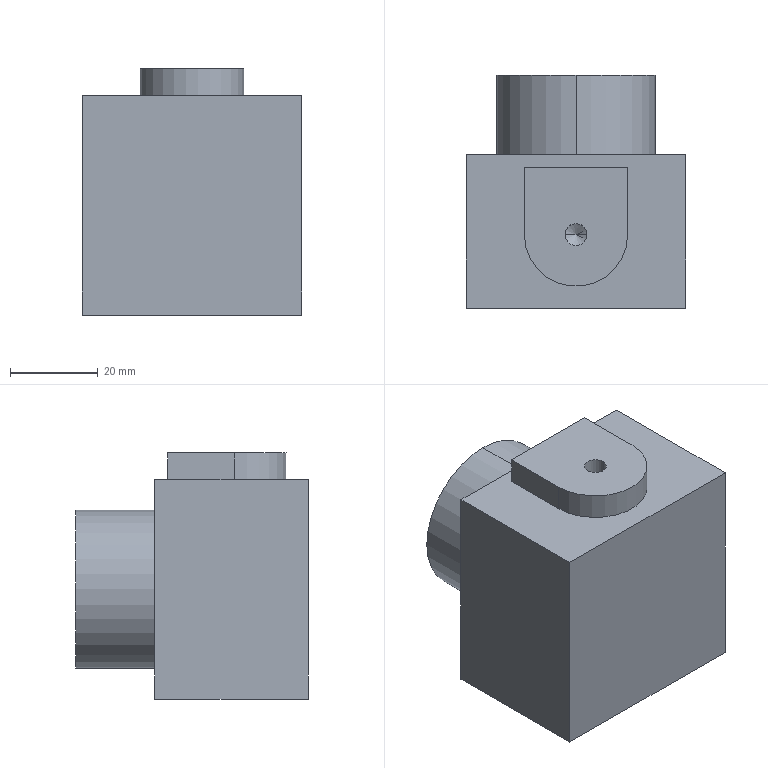Part | SolidWorks | features ICE 2, Extrusion 1, HoleWzd 1 | 1 solid | 18 faces | box 50 x 53 x 56 mm | volume 108930 mm3 | plane 11 | cylinder 5 | cone 2 | commonest cylinder face diameters 5 x2 36 x2 23.5 x1
STEP:
#1=CARTESIAN_POINT('',(-2.5,16.75,14.));
#2=VERTEX_POINT('',#1);
#3=CARTESIAN_POINT('',(2.5,16.75,14.));
#4=VERTEX_POINT('',#3);
#5=CARTESIAN_POINT('',(0.,16.75,14.));
#6=DIRECTION('',(0.,0.,1.));
#7=DIRECTION('',(1.,0.,0.));
#8=AXIS2_PLACEMENT_3D('',#5,#6,#7);
#9=CIRCLE('',#8,2.5);
#10=EDGE_CURVE('',#2,#4,#9,.T.);
#11=ORIENTED_EDGE('',*,*,#10,.F.);
#12=CARTESIAN_POINT('',(-2.5,16.75,31.));
#13=VERTEX_POINT('',#12);
#14=CARTESIAN_POINT('',(-2.5,16.75,31.));
#15=DIRECTION('',(0.,0.,1.));
#16=VECTOR('',#15,1000.);
#17=LINE('',#14,#16);
#18=EDGE_CURVE('',#2,#13,#17,.T.);
#19=ORIENTED_EDGE('',*,*,#18,.T.);
#20=CARTESIAN_POINT('',(2.5,16.75,31.));
#21=VERTEX_POINT('',#20);
#22=CARTESIAN_POINT('',(0.,16.75,31.));
#23=DIRECTION('',(0.,0.,1.));
#24=DIRECTION('',(1.,0.,0.));
#25=AXIS2_PLACEMENT_3D('',#22,#23,#24);
#26=CIRCLE('',#25,2.5);
#27=EDGE_CURVE('',#13,#21,#26,.T.);
#28=ORIENTED_EDGE('',*,*,#27,.T.);
#29=CARTESIAN_POINT('',(2.5,16.75,31.));
#30=DIRECTION('',(0.,0.,1.));
#31=VECTOR('',#30,1000.);
#32=LINE('',#29,#31);
#33=EDGE_CURVE('',#4,#21,#32,.T.);
#34=ORIENTED_EDGE('',*,*,#33,.F.);
#35=EDGE_LOOP('',(#11,#19,#28,#34));
#36=FACE_OUTER_BOUND('',#35,.T.);
#37=CARTESIAN_POINT('',(0.,16.75,31.));
#38=DIRECTION('',(0.,0.,1.));
#39=DIRECTION('',(1.,0.,0.));
#40=AXIS2_PLACEMENT_3D('',#37,#38,#39);
#41=CYLINDRICAL_SURFACE('',#40,2.5);
#42=ADVANCED_FACE('',(#36),#41,.F.);
#43=CARTESIAN_POINT('',(0.,16.75,12.498));
#44=VERTEX_POINT('',#43);
#45=CARTESIAN_POINT('',(2.5,16.75,14.));
#46=DIRECTION('',(0.8572,0.,0.515));
#47=VECTOR('',#46,1000.);
#48=LINE('',#45,#47);
#49=EDGE_CURVE('',#44,#4,#48,.T.);
#50=ORIENTED_EDGE('',*,*,#49,.F.);
#51=CARTESIAN_POINT('',(-2.5,16.75,14.));
#52=DIRECTION('',(-0.8572,0.,0.515));
#53=VECTOR('',#52,1000.);
#54=LINE('',#51,#53);
#55=EDGE_CURVE('',#44,#2,#54,.T.);
#56=ORIENTED_EDGE('',*,*,#55,.T.);
#57=ORIENTED_EDGE('',*,*,#10,.T.);
#58=EDGE_LOOP('',(#50,#56,#57));
#59=FACE_OUTER_BOUND('',#58,.T.);
#60=CARTESIAN_POINT('',(0.,16.75,14.));
#61=DIRECTION('',(0.,0.,1.));
#62=DIRECTION('',(1.,0.,0.));
#63=AXIS2_PLACEMENT_3D('',#60,#61,#62);
#64=CONICAL_SURFACE('',#63,2.5,1.03);
#65=ADVANCED_FACE('',(#59),#64,.F.);
#66=CARTESIAN_POINT('',(0.,53.,18.));
#67=VERTEX_POINT('',#66);
#68=CARTESIAN_POINT('',(0.,53.,-18.));
#69=VERTEX_POINT('',#68);
#70=CARTESIAN_POINT('',(0.,53.,0.));
#71=DIRECTION('',(0.,1.,0.));
#72=DIRECTION('',(0.,0.,1.));
#73=AXIS2_PLACEMENT_3D('',#70,#71,#72);
#74=CIRCLE('',#73,18.);
#75=EDGE_CURVE('',#67,#69,#74,.T.);
#76=ORIENTED_EDGE('',*,*,#75,.F.);
#77=CARTESIAN_POINT('',(0.,35.,18.));
#78=VERTEX_POINT('',#77);
#79=CARTESIAN_POINT('',(0.,53.,18.));
#80=DIRECTION('',(0.,-1.,0.));
#81=VECTOR('',#80,1000.);
#82=LINE('',#79,#81);
#83=EDGE_CURVE('',#67,#78,#82,.T.);
#84=ORIENTED_EDGE('',*,*,#83,.T.);
#85=CARTESIAN_POINT('',(0.,35.,-18.));
#86=VERTEX_POINT('',#85);
#87=CARTESIAN_POINT('',(0.,35.,0.));
#88=DIRECTION('',(0.,1.,0.));
#89=DIRECTION('',(0.,0.,1.));
#90=AXIS2_PLACEMENT_3D('',#87,#88,#89);
#91=CIRCLE('',#90,18.);
#92=EDGE_CURVE('',#78,#86,#91,.T.);
#93=ORIENTED_EDGE('',*,*,#92,.T.);
#94=CARTESIAN_POINT('',(0.,53.,-18.));
#95=DIRECTION('',(0.,-1.,0.));
#96=VECTOR('',#95,1000.);
#97=LINE('',#94,#96);
#98=EDGE_CURVE('',#69,#86,#97,.T.);
#99=ORIENTED_EDGE('',*,*,#98,.F.);
#100=EDGE_LOOP('',(#76,#84,#93,#99));
#101=FACE_OUTER_BOUND('',#100,.T.);
#102=CARTESIAN_POINT('',(0.,53.,0.));
#103=DIRECTION('',(0.,-1.,0.));
#104=DIRECTION('',(0.,0.,-1.));
#105=AXIS2_PLACEMENT_3D('',#102,#103,#104);
#106=CYLINDRICAL_SURFACE('',#105,18.);
#107=ADVANCED_FACE('',(#101),#106,.T.);
#108=CARTESIAN_POINT('',(-25.,0.,25.));
#109=VERTEX_POINT('',#108);
#110=CARTESIAN_POINT('',(25.,0.,25.));
#111=VERTEX_POINT('',#110);
#112=CARTESIAN_POINT('',(-25.,0.,25.));
#113=DIRECTION('',(1.,0.,0.));
#114=VECTOR('',#113,1000.);
#115=LINE('',#112,#114);
#116=EDGE_CURVE('',#109,#111,#115,.T.);
#117=ORIENTED_EDGE('',*,*,#116,.T.);
#118=CARTESIAN_POINT('',(25.,35.,25.));
#119=VERTEX_POINT('',#118);
#120=CARTESIAN_POINT('',(25.,35.,25.));
#121=DIRECTION('',(0.,-1.,0.));
#122=VECTOR('',#121,1000.);
#123=LINE('',#120,#122);
#124=EDGE_CURVE('',#119,#111,#123,.T.);
#125=ORIENTED_EDGE('',*,*,#124,.F.);
#126=CARTESIAN_POINT('',(-25.,35.,25.));
#127=VERTEX_POINT('',#126);
#128=CARTESIAN_POINT('',(-25.,35.,25.));
#129=DIRECTION('',(1.,0.,0.));
#130=VECTOR('',#129,1000.);
#131=LINE('',#128,#130);
#132=EDGE_CURVE('',#127,#119,#131,.T.);
#133=ORIENTED_EDGE('',*,*,#132,.F.);
#134=CARTESIAN_POINT('',(-25.,35.,25.));
#135=DIRECTION('',(0.,-1.,0.));
#136=VECTOR('',#135,1000.);
#137=LINE('',#134,#136);
#138=EDGE_CURVE('',#127,#109,#137,.T.);
#139=ORIENTED_EDGE('',*,*,#138,.T.);
#140=EDGE_LOOP('',(#117,#125,#133,#139));
#141=FACE_OUTER_BOUND('',#140,.T.);
#142=CARTESIAN_POINT('',(-11.75,16.75,25.));
#143=VERTEX_POINT('',#142);
#144=CARTESIAN_POINT('',(11.75,16.75,25.));
#145=VERTEX_POINT('',#144);
#146=CARTESIAN_POINT('',(0.,16.75,25.));
#147=DIRECTION('',(0.,0.,1.));
#148=DIRECTION('',(-1.,0.,0.));
#149=AXIS2_PLACEMENT_3D('',#146,#147,#148);
#150=CIRCLE('',#149,11.75);
#151=EDGE_CURVE('',#143,#145,#150,.T.);
#152=ORIENTED_EDGE('',*,*,#151,.F.);
#153=CARTESIAN_POINT('',(-11.75,32.,25.));
#154=VERTEX_POINT('',#153);
#155=CARTESIAN_POINT('',(-11.75,32.,25.));
#156=DIRECTION('',(0.,-1.,0.));
#157=VECTOR('',#156,1000.);
#158=LINE('',#155,#157);
#159=EDGE_CURVE('',#154,#143,#158,.T.);
#160=ORIENTED_EDGE('',*,*,#159,.F.);
#161=CARTESIAN_POINT('',(11.75,32.,25.));
#162=VERTEX_POINT('',#161);
#163=CARTESIAN_POINT('',(11.75,32.,25.));
#164=DIRECTION('',(-1.,0.,0.));
#165=VECTOR('',#164,1000.);
#166=LINE('',#163,#165);
#167=EDGE_CURVE('',#162,#154,#166,.T.);
#168=ORIENTED_EDGE('',*,*,#167,.F.);
#169=CARTESIAN_POINT('',(11.75,32.,25.));
#170=DIRECTION('',(0.,1.,0.));
#171=VECTOR('',#170,1000.);
#172=LINE('',#169,#171);
#173=EDGE_CURVE('',#145,#162,#172,.T.);
#174=ORIENTED_EDGE('',*,*,#173,.F.);
#175=EDGE_LOOP('',(#152,#160,#168,#174));
#176=FACE_BOUND('',#175,.T.);
#177=CARTESIAN_POINT('',(-25.,35.,25.));
#178=DIRECTION('',(0.,0.,-1.));
#179=DIRECTION('',(-1.,0.,0.));
#180=AXIS2_PLACEMENT_3D('',#177,#178,#179);
#181=PLANE('',#180);
#182=ADVANCED_FACE('',(#141,#176),#181,.F.);
#183=CARTESIAN_POINT('',(25.,0.,-25.));
#184=VERTEX_POINT('',#183);
#185=CARTESIAN_POINT('',(25.,0.,25.));
#186=DIRECTION('',(0.,0.,-1.));
#187=VECTOR('',#186,1000.);
#188=LINE('',#185,#187);
#189=EDGE_CURVE('',#111,#184,#188,.T.);
#190=ORIENTED_EDGE('',*,*,#189,.T.);
#191=CARTESIAN_POINT('',(25.,35.,-25.));
#192=VERTEX_POINT('',#191);
#193=CARTESIAN_POINT('',(25.,35.,-25.));
#194=DIRECTION('',(0.,-1.,0.));
#195=VECTOR('',#194,1000.);
#196=LINE('',#193,#195);
#197=EDGE_CURVE('',#192,#184,#196,.T.);
#198=ORIENTED_EDGE('',*,*,#197,.F.);
#199=CARTESIAN_POINT('',(25.,35.,25.));
#200=DIRECTION('',(0.,0.,-1.));
#201=VECTOR('',#200,1000.);
#202=LINE('',#199,#201);
#203=EDGE_CURVE('',#119,#192,#202,.T.);
#204=ORIENTED_EDGE('',*,*,#203,.F.);
#205=ORIENTED_EDGE('',*,*,#124,.T.);
#206=EDGE_LOOP('',(#190,#198,#204,#205));
#207=FACE_OUTER_BOUND('',#206,.T.);
#208=CARTESIAN_POINT('',(25.,35.,25.));
#209=DIRECTION('',(-1.,0.,0.));
#210=DIRECTION('',(0.,0.,1.));
#211=AXIS2_PLACEMENT_3D('',#208,#209,#210);
#212=PLANE('',#211);
#213=ADVANCED_FACE('',(#207),#212,.F.);
#214=CARTESIAN_POINT('',(-25.,0.,-25.));
#215=VERTEX_POINT('',#214);
#216=CARTESIAN_POINT('',(-25.,0.,-25.));
#217=DIRECTION('',(-1.,0.,0.));
#218=VECTOR('',#217,1000.);
#219=LINE('',#216,#218);
#220=EDGE_CURVE('',#184,#215,#219,.T.);
#221=ORIENTED_EDGE('',*,*,#220,.T.);
#222=CARTESIAN_POINT('',(-25.,35.,-25.));
#223=VERTEX_POINT('',#222);
#224=CARTESIAN_POINT('',(-25.,35.,-25.));
#225=DIRECTION('',(0.,-1.,0.));
#226=VECTOR('',#225,1000.);
#227=LINE('',#224,#226);
#228=EDGE_CURVE('',#223,#215,#227,.T.);
#229=ORIENTED_EDGE('',*,*,#228,.F.);
#230=CARTESIAN_POINT('',(-25.,35.,-25.));
#231=DIRECTION('',(-1.,0.,0.));
#232=VECTOR('',#231,1000.);
#233=LINE('',#230,#232);
#234=EDGE_CURVE('',#192,#223,#233,.T.);
#235=ORIENTED_EDGE('',*,*,#234,.F.);
#236=ORIENTED_EDGE('',*,*,#197,.T.);
#237=EDGE_LOOP('',(#221,#229,#235,#236));
#238=FACE_OUTER_BOUND('',#237,.T.);
#239=CARTESIAN_POINT('',(-25.,35.,-25.));
#240=DIRECTION('',(0.,0.,1.));
#241=DIRECTION('',(1.,0.,0.));
#242=AXIS2_PLACEMENT_3D('',#239,#240,#241);
#243=PLANE('',#242);
#244=ADVANCED_FACE('',(#238),#243,.F.);
#245=CARTESIAN_POINT('',(-25.,0.,25.));
#246=DIRECTION('',(0.,0.,1.));
#247=VECTOR('',#246,1000.);
#248=LINE('',#245,#247);
#249=EDGE_CURVE('',#215,#109,#248,.T.);
#250=ORIENTED_EDGE('',*,*,#249,.T.);
#251=ORIENTED_EDGE('',*,*,#138,.F.);
#252=CARTESIAN_POINT('',(-25.,35.,25.));
#253=DIRECTION('',(0.,0.,1.));
#254=VECTOR('',#253,1000.);
#255=LINE('',#252,#254);
#256=EDGE_CURVE('',#223,#127,#255,.T.);
#257=ORIENTED_EDGE('',*,*,#256,.F.);
#258=ORIENTED_EDGE('',*,*,#228,.T.);
#259=EDGE_LOOP('',(#250,#251,#257,#258));
#260=FACE_OUTER_BOUND('',#259,.T.);
#261=CARTESIAN_POINT('',(-25.,35.,25.));
#262=DIRECTION('',(1.,0.,0.));
#263=DIRECTION('',(0.,0.,-1.));
#264=AXIS2_PLACEMENT_3D('',#261,#262,#263);
#265=PLANE('',#264);
#266=ADVANCED_FACE('',(#260),#265,.F.);
#267=CARTESIAN_POINT('',(0.,35.,0.));
#268=DIRECTION('',(0.,1.,0.));
#269=DIRECTION('',(0.,0.,1.));
#270=AXIS2_PLACEMENT_3D('',#267,#268,#269);
#271=CIRCLE('',#270,18.);
#272=EDGE_CURVE('',#86,#78,#271,.T.);
#273=ORIENTED_EDGE('',*,*,#272,.F.);
#274=ORIENTED_EDGE('',*,*,#92,.F.);
#275=EDGE_LOOP('',(#273,#274));
#276=FACE_BOUND('',#275,.T.);
#277=ORIENTED_EDGE('',*,*,#203,.T.);
#278=ORIENTED_EDGE('',*,*,#234,.T.);
#279=ORIENTED_EDGE('',*,*,#256,.T.);
#280=ORIENTED_EDGE('',*,*,#132,.T.);
#281=EDGE_LOOP('',(#277,#278,#279,#280));
#282=FACE_OUTER_BOUND('',#281,.T.);
#283=CARTESIAN_POINT('',(0.,35.,0.));
#284=DIRECTION('',(0.,-1.,0.));
#285=DIRECTION('',(0.,0.,-1.));
#286=AXIS2_PLACEMENT_3D('',#283,#284,#285);
#287=PLANE('',#286);
#288=ADVANCED_FACE('',(#276,#282),#287,.F.);
#289=ORIENTED_EDGE('',*,*,#189,.F.);
#290=ORIENTED_EDGE('',*,*,#116,.F.);
#291=ORIENTED_EDGE('',*,*,#249,.F.);
#292=ORIENTED_EDGE('',*,*,#220,.F.);
#293=EDGE_LOOP('',(#289,#290,#291,#292));
#294=FACE_OUTER_BOUND('',#293,.T.);
#295=CARTESIAN_POINT('',(0.,0.,0.));
#296=DIRECTION('',(0.,-1.,0.));
#297=DIRECTION('',(0.,0.,-1.));
#298=AXIS2_PLACEMENT_3D('',#295,#296,#297);
#299=PLANE('',#298);
#300=ADVANCED_FACE('',(#294),#299,.T.);
#301=ORIENTED_EDGE('',*,*,#83,.F.);
#302=CARTESIAN_POINT('',(0.,53.,0.));
#303=DIRECTION('',(0.,1.,0.));
#304=DIRECTION('',(0.,0.,1.));
#305=AXIS2_PLACEMENT_3D('',#302,#303,#304);
#306=CIRCLE('',#305,18.);
#307=EDGE_CURVE('',#69,#67,#306,.T.);
#308=ORIENTED_EDGE('',*,*,#307,.F.);
#309=ORIENTED_EDGE('',*,*,#98,.T.);
#310=ORIENTED_EDGE('',*,*,#272,.T.);
#311=EDGE_LOOP('',(#301,#308,#309,#310));
#312=FACE_OUTER_BOUND('',#311,.T.);
#313=CARTESIAN_POINT('',(0.,53.,0.));
#314=DIRECTION('',(0.,-1.,0.));
#315=DIRECTION('',(0.,0.,-1.));
#316=AXIS2_PLACEMENT_3D('',#313,#314,#315);
#317=CYLINDRICAL_SURFACE('',#316,18.);
#318=ADVANCED_FACE('',(#312),#317,.T.);
#319=ORIENTED_EDGE('',*,*,#307,.T.);
#320=ORIENTED_EDGE('',*,*,#75,.T.);
#321=EDGE_LOOP('',(#319,#320));
#322=FACE_OUTER_BOUND('',#321,.T.);
#323=CARTESIAN_POINT('',(0.,53.,0.));
#324=DIRECTION('',(0.,1.,0.));
#325=DIRECTION('',(0.,0.,1.));
#326=AXIS2_PLACEMENT_3D('',#323,#324,#325);
#327=PLANE('',#326);
#328=ADVANCED_FACE('',(#322),#327,.T.);
#329=ORIENTED_EDGE('',*,*,#151,.T.);
#330=CARTESIAN_POINT('',(11.75,16.75,31.));
#331=VERTEX_POINT('',#330);
#332=CARTESIAN_POINT('',(11.75,16.75,31.));
#333=DIRECTION('',(0.,0.,-1.));
#334=VECTOR('',#333,1000.);
#335=LINE('',#332,#334);
#336=EDGE_CURVE('',#331,#145,#335,.T.);
#337=ORIENTED_EDGE('',*,*,#336,.F.);
#338=CARTESIAN_POINT('',(-11.75,16.75,31.));
#339=VERTEX_POINT('',#338);
#340=CARTESIAN_POINT('',(0.,16.75,31.));
#341=DIRECTION('',(0.,0.,1.));
#342=DIRECTION('',(-1.,0.,0.));
#343=AXIS2_PLACEMENT_3D('',#340,#341,#342);
#344=CIRCLE('',#343,11.75);
#345=EDGE_CURVE('',#339,#331,#344,.T.);
#346=ORIENTED_EDGE('',*,*,#345,.F.);
#347=CARTESIAN_POINT('',(-11.75,16.75,31.));
#348=DIRECTION('',(0.,0.,-1.));
#349=VECTOR('',#348,1000.);
#350=LINE('',#347,#349);
#351=EDGE_CURVE('',#339,#143,#350,.T.);
#352=ORIENTED_EDGE('',*,*,#351,.T.);
#353=EDGE_LOOP('',(#329,#337,#346,#352));
#354=FACE_OUTER_BOUND('',#353,.T.);
#355=CARTESIAN_POINT('',(0.,16.75,31.));
#356=DIRECTION('',(0.,0.,-1.));
#357=DIRECTION('',(-1.,0.,0.));
#358=AXIS2_PLACEMENT_3D('',#355,#356,#357);
#359=CYLINDRICAL_SURFACE('',#358,11.75);
#360=ADVANCED_FACE('',(#354),#359,.T.);
#361=ORIENTED_EDGE('',*,*,#173,.T.);
#362=CARTESIAN_POINT('',(11.75,32.,31.));
#363=VERTEX_POINT('',#362);
#364=CARTESIAN_POINT('',(11.75,32.,31.));
#365=DIRECTION('',(0.,0.,-1.));
#366=VECTOR('',#365,1000.);
#367=LINE('',#364,#366);
#368=EDGE_CURVE('',#363,#162,#367,.T.);
#369=ORIENTED_EDGE('',*,*,#368,.F.);
#370=CARTESIAN_POINT('',(11.75,32.,31.));
#371=DIRECTION('',(0.,1.,0.));
#372=VECTOR('',#371,1000.);
#373=LINE('',#370,#372);
#374=EDGE_CURVE('',#331,#363,#373,.T.);
#375=ORIENTED_EDGE('',*,*,#374,.F.);
#376=ORIENTED_EDGE('',*,*,#336,.T.);
#377=EDGE_LOOP('',(#361,#369,#375,#376));
#378=FACE_OUTER_BOUND('',#377,.T.);
#379=CARTESIAN_POINT('',(11.75,32.,31.));
#380=DIRECTION('',(-1.,0.,0.));
#381=DIRECTION('',(0.,-1.,0.));
#382=AXIS2_PLACEMENT_3D('',#379,#380,#381);
#383=PLANE('',#382);
#384=ADVANCED_FACE('',(#378),#383,.F.);
#385=ORIENTED_EDGE('',*,*,#167,.T.);
#386=CARTESIAN_POINT('',(-11.75,32.,31.));
#387=VERTEX_POINT('',#386);
#388=CARTESIAN_POINT('',(-11.75,32.,31.));
#389=DIRECTION('',(0.,0.,-1.));
#390=VECTOR('',#389,1000.);
#391=LINE('',#388,#390);
#392=EDGE_CURVE('',#387,#154,#391,.T.);
#393=ORIENTED_EDGE('',*,*,#392,.F.);
#394=CARTESIAN_POINT('',(11.75,32.,31.));
#395=DIRECTION('',(-1.,0.,0.));
#396=VECTOR('',#395,1000.);
#397=LINE('',#394,#396);
#398=EDGE_CURVE('',#363,#387,#397,.T.);
#399=ORIENTED_EDGE('',*,*,#398,.F.);
#400=ORIENTED_EDGE('',*,*,#368,.T.);
#401=EDGE_LOOP('',(#385,#393,#399,#400));
#402=FACE_OUTER_BOUND('',#401,.T.);
#403=CARTESIAN_POINT('',(11.75,32.,31.));
#404=DIRECTION('',(0.,-1.,0.));
#405=DIRECTION('',(0.,0.,-1.));
#406=AXIS2_PLACEMENT_3D('',#403,#404,#405);
#407=PLANE('',#406);
#408=ADVANCED_FACE('',(#402),#407,.F.);
#409=ORIENTED_EDGE('',*,*,#159,.T.);
#410=ORIENTED_EDGE('',*,*,#351,.F.);
#411=CARTESIAN_POINT('',(-11.75,32.,31.));
#412=DIRECTION('',(0.,-1.,0.));
#413=VECTOR('',#412,1000.);
#414=LINE('',#411,#413);
#415=EDGE_CURVE('',#387,#339,#414,.T.);
#416=ORIENTED_EDGE('',*,*,#415,.F.);
#417=ORIENTED_EDGE('',*,*,#392,.T.);
#418=EDGE_LOOP('',(#409,#410,#416,#417));
#419=FACE_OUTER_BOUND('',#418,.T.);
#420=CARTESIAN_POINT('',(-11.75,32.,31.));
#421=DIRECTION('',(1.,0.,0.));
#422=DIRECTION('',(0.,1.,0.));
#423=AXIS2_PLACEMENT_3D('',#420,#421,#422);
#424=PLANE('',#423);
#425=ADVANCED_FACE('',(#419),#424,.F.);
#426=CARTESIAN_POINT('',(0.,16.75,31.));
#427=DIRECTION('',(0.,0.,1.));
#428=DIRECTION('',(1.,0.,0.));
#429=AXIS2_PLACEMENT_3D('',#426,#427,#428);
#430=CIRCLE('',#429,2.5);
#431=EDGE_CURVE('',#21,#13,#430,.T.);
#432=ORIENTED_EDGE('',*,*,#431,.F.);
#433=ORIENTED_EDGE('',*,*,#27,.F.);
#434=EDGE_LOOP('',(#432,#433));
#435=FACE_BOUND('',#434,.T.);
#436=ORIENTED_EDGE('',*,*,#345,.T.);
#437=ORIENTED_EDGE('',*,*,#374,.T.);
#438=ORIENTED_EDGE('',*,*,#398,.T.);
#439=ORIENTED_EDGE('',*,*,#415,.T.);
#440=EDGE_LOOP('',(#436,#437,#438,#439));
#441=FACE_OUTER_BOUND('',#440,.T.);
#442=CARTESIAN_POINT('',(0.,16.75,31.));
#443=DIRECTION('',(0.,0.,-1.));
#444=DIRECTION('',(-1.,0.,0.));
#445=AXIS2_PLACEMENT_3D('',#442,#443,#444);
#446=PLANE('',#445);
#447=ADVANCED_FACE('',(#435,#441),#446,.F.);
#448=ORIENTED_EDGE('',*,*,#55,.F.);
#449=ORIENTED_EDGE('',*,*,#49,.T.);
#450=CARTESIAN_POINT('',(0.,16.75,14.));
#451=DIRECTION('',(0.,0.,1.));
#452=DIRECTION('',(1.,0.,0.));
#453=AXIS2_PLACEMENT_3D('',#450,#451,#452);
#454=CIRCLE('',#453,2.5);
#455=EDGE_CURVE('',#4,#2,#454,.T.);
#456=ORIENTED_EDGE('',*,*,#455,.T.);
#457=EDGE_LOOP('',(#448,#449,#456));
#458=FACE_OUTER_BOUND('',#457,.T.);
#459=CARTESIAN_POINT('',(0.,16.75,14.));
#460=DIRECTION('',(0.,0.,1.));
#461=DIRECTION('',(1.,0.,0.));
#462=AXIS2_PLACEMENT_3D('',#459,#460,#461);
#463=CONICAL_SURFACE('',#462,2.5,1.03);
#464=ADVANCED_FACE('',(#458),#463,.F.);
#465=ORIENTED_EDGE('',*,*,#18,.F.);
#466=ORIENTED_EDGE('',*,*,#455,.F.);
#467=ORIENTED_EDGE('',*,*,#33,.T.);
#468=ORIENTED_EDGE('',*,*,#431,.T.);
#469=EDGE_LOOP('',(#465,#466,#467,#468));
#470=FACE_OUTER_BOUND('',#469,.T.);
#471=CARTESIAN_POINT('',(0.,16.75,31.));
#472=DIRECTION('',(0.,0.,1.));
#473=DIRECTION('',(1.,0.,0.));
#474=AXIS2_PLACEMENT_3D('',#471,#472,#473);
#475=CYLINDRICAL_SURFACE('',#474,2.5);
#476=ADVANCED_FACE('',(#470),#475,.F.);
#477=CLOSED_SHELL('',(#42,#65,#107,#182,#213,#244,#266,#288,#300,#318,#328,#360,#384,#408,#425,#447,#464,#476));
#478=MANIFOLD_SOLID_BREP('',#477);
#479=CARTESIAN_POINT('',(0.,0.,0.));
#480=DIRECTION('',(0.,0.,1.));
#481=DIRECTION('',(1.,0.,0.));
#482=AXIS2_PLACEMENT_3D('',#479,#480,#481);
#483=(LENGTH_UNIT()NAMED_UNIT(*)SI_UNIT(.MILLI.,.METRE.));
#484=UNCERTAINTY_MEASURE_WITH_UNIT(LENGTH_MEASURE(0.00001),#483,'','');
#485=(NAMED_UNIT(*)PLANE_ANGLE_UNIT()SI_UNIT($,.RADIAN.));
#486=(NAMED_UNIT(*)SI_UNIT($,.STERADIAN.)SOLID_ANGLE_UNIT());
#487=(GEOMETRIC_REPRESENTATION_CONTEXT(3)GLOBAL_UNCERTAINTY_ASSIGNED_CONTEXT((#484))GLOBAL_UNIT_ASSIGNED_CONTEXT((#483,#485,#486))REPRESENTATION_CONTEXT('',''));
#488=ADVANCED_BREP_SHAPE_REPRESENTATION('',(#478,#482),#487);